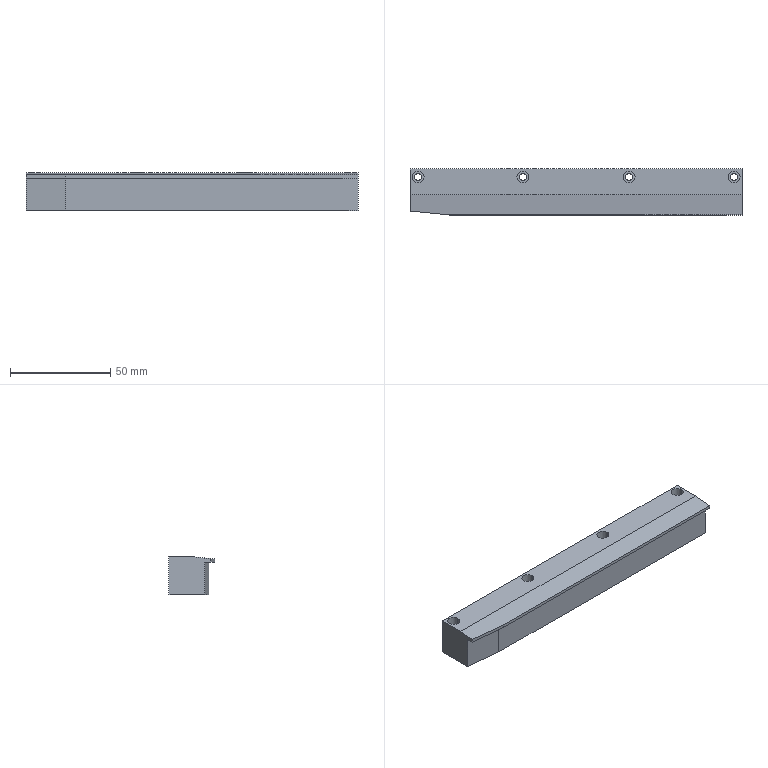Part | SolidWorks | features BaseBody 1 | 1 solid | 31 faces | box 166 x 23 x 19 mm | volume 61656 mm3 | cylinder 16 | plane 15 | commonest cylinder face diameters 3.5 x8 6 x8
STEP:
#1=CARTESIAN_POINT('',(-20.019,-11.953,0.));
#2=VERTEX_POINT('',#1);
#3=CARTESIAN_POINT('',(-23.519,-11.953,0.));
#4=VERTEX_POINT('',#3);
#5=CARTESIAN_POINT('',(-21.769,-11.953,0.));
#6=DIRECTION('',(0.,0.,-1.));
#7=DIRECTION('',(1.,0.,0.));
#8=AXIS2_PLACEMENT_3D('',#5,#6,#7);
#9=CIRCLE('',#8,1.75);
#10=EDGE_CURVE('',#2,#4,#9,.T.);
#11=ORIENTED_EDGE('',*,*,#10,.T.);
#12=CARTESIAN_POINT('',(-23.519,-11.953,9.));
#13=VERTEX_POINT('',#12);
#14=CARTESIAN_POINT('',(-23.519,-11.953,-149.799));
#15=DIRECTION('',(0.,0.,1.));
#16=VECTOR('',#15,1000.);
#17=LINE('',#14,#16);
#18=EDGE_CURVE('',#4,#13,#17,.T.);
#19=ORIENTED_EDGE('',*,*,#18,.T.);
#20=CARTESIAN_POINT('',(-20.019,-11.953,9.));
#21=VERTEX_POINT('',#20);
#22=CARTESIAN_POINT('',(-21.769,-11.953,9.));
#23=DIRECTION('',(0.,0.,-1.));
#24=DIRECTION('',(1.,0.,0.));
#25=AXIS2_PLACEMENT_3D('',#22,#23,#24);
#26=CIRCLE('',#25,1.75);
#27=EDGE_CURVE('',#21,#13,#26,.T.);
#28=ORIENTED_EDGE('',*,*,#27,.F.);
#29=CARTESIAN_POINT('',(-20.019,-11.953,-149.799));
#30=DIRECTION('',(0.,0.,1.));
#31=VECTOR('',#30,1000.);
#32=LINE('',#29,#31);
#33=EDGE_CURVE('',#2,#21,#32,.T.);
#34=ORIENTED_EDGE('',*,*,#33,.F.);
#35=EDGE_LOOP('',(#11,#19,#28,#34));
#36=FACE_OUTER_BOUND('',#35,.T.);
#37=CARTESIAN_POINT('',(-21.769,-11.953,-149.799));
#38=DIRECTION('',(0.,0.,1.));
#39=DIRECTION('',(1.,0.,0.));
#40=AXIS2_PLACEMENT_3D('',#37,#38,#39);
#41=CYLINDRICAL_SURFACE('',#40,1.75);
#42=ADVANCED_FACE('',(#36),#41,.F.);
#43=CARTESIAN_POINT('',(32.481,-11.953,0.));
#44=VERTEX_POINT('',#43);
#45=CARTESIAN_POINT('',(28.981,-11.953,0.));
#46=VERTEX_POINT('',#45);
#47=CARTESIAN_POINT('',(30.731,-11.953,0.));
#48=DIRECTION('',(0.,0.,-1.));
#49=DIRECTION('',(1.,0.,0.));
#50=AXIS2_PLACEMENT_3D('',#47,#48,#49);
#51=CIRCLE('',#50,1.75);
#52=EDGE_CURVE('',#44,#46,#51,.T.);
#53=ORIENTED_EDGE('',*,*,#52,.T.);
#54=CARTESIAN_POINT('',(28.981,-11.953,9.));
#55=VERTEX_POINT('',#54);
#56=CARTESIAN_POINT('',(28.981,-11.953,-149.799));
#57=DIRECTION('',(0.,0.,1.));
#58=VECTOR('',#57,1000.);
#59=LINE('',#56,#58);
#60=EDGE_CURVE('',#46,#55,#59,.T.);
#61=ORIENTED_EDGE('',*,*,#60,.T.);
#62=CARTESIAN_POINT('',(32.481,-11.953,9.));
#63=VERTEX_POINT('',#62);
#64=CARTESIAN_POINT('',(30.731,-11.953,9.));
#65=DIRECTION('',(0.,0.,-1.));
#66=DIRECTION('',(1.,0.,0.));
#67=AXIS2_PLACEMENT_3D('',#64,#65,#66);
#68=CIRCLE('',#67,1.75);
#69=EDGE_CURVE('',#63,#55,#68,.T.);
#70=ORIENTED_EDGE('',*,*,#69,.F.);
#71=CARTESIAN_POINT('',(32.481,-11.953,-149.799));
#72=DIRECTION('',(0.,0.,1.));
#73=VECTOR('',#72,1000.);
#74=LINE('',#71,#73);
#75=EDGE_CURVE('',#44,#63,#74,.T.);
#76=ORIENTED_EDGE('',*,*,#75,.F.);
#77=EDGE_LOOP('',(#53,#61,#70,#76));
#78=FACE_OUTER_BOUND('',#77,.T.);
#79=CARTESIAN_POINT('',(30.731,-11.953,-149.799));
#80=DIRECTION('',(0.,0.,1.));
#81=DIRECTION('',(1.,0.,0.));
#82=AXIS2_PLACEMENT_3D('',#79,#80,#81);
#83=CYLINDRICAL_SURFACE('',#82,1.75);
#84=ADVANCED_FACE('',(#78),#83,.F.);
#85=CARTESIAN_POINT('',(85.481,-11.953,0.));
#86=VERTEX_POINT('',#85);
#87=CARTESIAN_POINT('',(81.981,-11.953,0.));
#88=VERTEX_POINT('',#87);
#89=CARTESIAN_POINT('',(83.731,-11.953,0.));
#90=DIRECTION('',(0.,0.,-1.));
#91=DIRECTION('',(1.,0.,0.));
#92=AXIS2_PLACEMENT_3D('',#89,#90,#91);
#93=CIRCLE('',#92,1.75);
#94=EDGE_CURVE('',#86,#88,#93,.T.);
#95=ORIENTED_EDGE('',*,*,#94,.T.);
#96=CARTESIAN_POINT('',(81.981,-11.953,9.));
#97=VERTEX_POINT('',#96);
#98=CARTESIAN_POINT('',(81.981,-11.953,-149.799));
#99=DIRECTION('',(0.,0.,1.));
#100=VECTOR('',#99,1000.);
#101=LINE('',#98,#100);
#102=EDGE_CURVE('',#88,#97,#101,.T.);
#103=ORIENTED_EDGE('',*,*,#102,.T.);
#104=CARTESIAN_POINT('',(85.481,-11.953,9.));
#105=VERTEX_POINT('',#104);
#106=CARTESIAN_POINT('',(83.731,-11.953,9.));
#107=DIRECTION('',(0.,0.,-1.));
#108=DIRECTION('',(1.,0.,0.));
#109=AXIS2_PLACEMENT_3D('',#106,#107,#108);
#110=CIRCLE('',#109,1.75);
#111=EDGE_CURVE('',#105,#97,#110,.T.);
#112=ORIENTED_EDGE('',*,*,#111,.F.);
#113=CARTESIAN_POINT('',(85.481,-11.953,-149.799));
#114=DIRECTION('',(0.,0.,1.));
#115=VECTOR('',#114,1000.);
#116=LINE('',#113,#115);
#117=EDGE_CURVE('',#86,#105,#116,.T.);
#118=ORIENTED_EDGE('',*,*,#117,.F.);
#119=EDGE_LOOP('',(#95,#103,#112,#118));
#120=FACE_OUTER_BOUND('',#119,.T.);
#121=CARTESIAN_POINT('',(83.731,-11.953,-149.799));
#122=DIRECTION('',(0.,0.,1.));
#123=DIRECTION('',(1.,0.,0.));
#124=AXIS2_PLACEMENT_3D('',#121,#122,#123);
#125=CYLINDRICAL_SURFACE('',#124,1.75);
#126=ADVANCED_FACE('',(#120),#125,.F.);
#127=CARTESIAN_POINT('',(137.981,-11.953,0.));
#128=VERTEX_POINT('',#127);
#129=CARTESIAN_POINT('',(134.481,-11.953,0.));
#130=VERTEX_POINT('',#129);
#131=CARTESIAN_POINT('',(136.231,-11.953,0.));
#132=DIRECTION('',(0.,0.,-1.));
#133=DIRECTION('',(1.,0.,0.));
#134=AXIS2_PLACEMENT_3D('',#131,#132,#133);
#135=CIRCLE('',#134,1.75);
#136=EDGE_CURVE('',#128,#130,#135,.T.);
#137=ORIENTED_EDGE('',*,*,#136,.T.);
#138=CARTESIAN_POINT('',(134.481,-11.953,9.));
#139=VERTEX_POINT('',#138);
#140=CARTESIAN_POINT('',(134.481,-11.953,-149.799));
#141=DIRECTION('',(0.,0.,1.));
#142=VECTOR('',#141,1000.);
#143=LINE('',#140,#142);
#144=EDGE_CURVE('',#130,#139,#143,.T.);
#145=ORIENTED_EDGE('',*,*,#144,.T.);
#146=CARTESIAN_POINT('',(137.981,-11.953,9.));
#147=VERTEX_POINT('',#146);
#148=CARTESIAN_POINT('',(136.231,-11.953,9.));
#149=DIRECTION('',(0.,0.,-1.));
#150=DIRECTION('',(1.,0.,0.));
#151=AXIS2_PLACEMENT_3D('',#148,#149,#150);
#152=CIRCLE('',#151,1.75);
#153=EDGE_CURVE('',#147,#139,#152,.T.);
#154=ORIENTED_EDGE('',*,*,#153,.F.);
#155=CARTESIAN_POINT('',(137.981,-11.953,-149.799));
#156=DIRECTION('',(0.,0.,1.));
#157=VECTOR('',#156,1000.);
#158=LINE('',#155,#157);
#159=EDGE_CURVE('',#128,#147,#158,.T.);
#160=ORIENTED_EDGE('',*,*,#159,.F.);
#161=EDGE_LOOP('',(#137,#145,#154,#160));
#162=FACE_OUTER_BOUND('',#161,.T.);
#163=CARTESIAN_POINT('',(136.231,-11.953,-149.799));
#164=DIRECTION('',(0.,0.,1.));
#165=DIRECTION('',(1.,0.,0.));
#166=AXIS2_PLACEMENT_3D('',#163,#164,#165);
#167=CYLINDRICAL_SURFACE('',#166,1.75);
#168=ADVANCED_FACE('',(#162),#167,.F.);
#169=CARTESIAN_POINT('',(-24.769,-11.953,9.));
#170=VERTEX_POINT('',#169);
#171=CARTESIAN_POINT('',(-18.769,-11.953,9.));
#172=VERTEX_POINT('',#171);
#173=CARTESIAN_POINT('',(-21.769,-11.953,9.));
#174=DIRECTION('',(0.,0.,1.));
#175=DIRECTION('',(1.,0.,0.));
#176=AXIS2_PLACEMENT_3D('',#173,#174,#175);
#177=CIRCLE('',#176,3.);
#178=EDGE_CURVE('',#170,#172,#177,.T.);
#179=ORIENTED_EDGE('',*,*,#178,.F.);
#180=CARTESIAN_POINT('',(-24.769,-11.953,19.));
#181=VERTEX_POINT('',#180);
#182=CARTESIAN_POINT('',(-24.769,-11.953,14.));
#183=DIRECTION('',(0.,0.,1.));
#184=VECTOR('',#183,1000.);
#185=LINE('',#182,#184);
#186=EDGE_CURVE('',#170,#181,#185,.T.);
#187=ORIENTED_EDGE('',*,*,#186,.T.);
#188=CARTESIAN_POINT('',(-18.769,-11.953,19.));
#189=VERTEX_POINT('',#188);
#190=CARTESIAN_POINT('',(-21.769,-11.953,19.));
#191=DIRECTION('',(0.,0.,-1.));
#192=DIRECTION('',(1.,0.,0.));
#193=AXIS2_PLACEMENT_3D('',#190,#191,#192);
#194=CIRCLE('',#193,3.);
#195=EDGE_CURVE('',#189,#181,#194,.T.);
#196=ORIENTED_EDGE('',*,*,#195,.F.);
#197=CARTESIAN_POINT('',(-18.769,-11.953,14.));
#198=DIRECTION('',(0.,0.,1.));
#199=VECTOR('',#198,1000.);
#200=LINE('',#197,#199);
#201=EDGE_CURVE('',#172,#189,#200,.T.);
#202=ORIENTED_EDGE('',*,*,#201,.F.);
#203=EDGE_LOOP('',(#179,#187,#196,#202));
#204=FACE_OUTER_BOUND('',#203,.T.);
#205=CARTESIAN_POINT('',(-21.769,-11.953,14.));
#206=DIRECTION('',(0.,0.,1.));
#207=DIRECTION('',(1.,0.,0.));
#208=AXIS2_PLACEMENT_3D('',#205,#206,#207);
#209=CYLINDRICAL_SURFACE('',#208,3.);
#210=ADVANCED_FACE('',(#204),#209,.F.);
#211=CARTESIAN_POINT('',(27.731,-11.953,9.));
#212=VERTEX_POINT('',#211);
#213=CARTESIAN_POINT('',(33.731,-11.953,9.));
#214=VERTEX_POINT('',#213);
#215=CARTESIAN_POINT('',(30.731,-11.953,9.));
#216=DIRECTION('',(0.,0.,1.));
#217=DIRECTION('',(1.,0.,0.));
#218=AXIS2_PLACEMENT_3D('',#215,#216,#217);
#219=CIRCLE('',#218,3.);
#220=EDGE_CURVE('',#212,#214,#219,.T.);
#221=ORIENTED_EDGE('',*,*,#220,.F.);
#222=CARTESIAN_POINT('',(27.731,-11.953,19.));
#223=VERTEX_POINT('',#222);
#224=CARTESIAN_POINT('',(27.731,-11.953,14.));
#225=DIRECTION('',(0.,0.,1.));
#226=VECTOR('',#225,1000.);
#227=LINE('',#224,#226);
#228=EDGE_CURVE('',#212,#223,#227,.T.);
#229=ORIENTED_EDGE('',*,*,#228,.T.);
#230=CARTESIAN_POINT('',(33.731,-11.953,19.));
#231=VERTEX_POINT('',#230);
#232=CARTESIAN_POINT('',(30.731,-11.953,19.));
#233=DIRECTION('',(0.,0.,-1.));
#234=DIRECTION('',(1.,0.,0.));
#235=AXIS2_PLACEMENT_3D('',#232,#233,#234);
#236=CIRCLE('',#235,3.);
#237=EDGE_CURVE('',#231,#223,#236,.T.);
#238=ORIENTED_EDGE('',*,*,#237,.F.);
#239=CARTESIAN_POINT('',(33.731,-11.953,14.));
#240=DIRECTION('',(0.,0.,1.));
#241=VECTOR('',#240,1000.);
#242=LINE('',#239,#241);
#243=EDGE_CURVE('',#214,#231,#242,.T.);
#244=ORIENTED_EDGE('',*,*,#243,.F.);
#245=EDGE_LOOP('',(#221,#229,#238,#244));
#246=FACE_OUTER_BOUND('',#245,.T.);
#247=CARTESIAN_POINT('',(30.731,-11.953,14.));
#248=DIRECTION('',(0.,0.,1.));
#249=DIRECTION('',(1.,0.,0.));
#250=AXIS2_PLACEMENT_3D('',#247,#248,#249);
#251=CYLINDRICAL_SURFACE('',#250,3.);
#252=ADVANCED_FACE('',(#246),#251,.F.);
#253=CARTESIAN_POINT('',(80.731,-11.953,9.));
#254=VERTEX_POINT('',#253);
#255=CARTESIAN_POINT('',(86.731,-11.953,9.));
#256=VERTEX_POINT('',#255);
#257=CARTESIAN_POINT('',(83.731,-11.953,9.));
#258=DIRECTION('',(0.,0.,1.));
#259=DIRECTION('',(1.,0.,0.));
#260=AXIS2_PLACEMENT_3D('',#257,#258,#259);
#261=CIRCLE('',#260,3.);
#262=EDGE_CURVE('',#254,#256,#261,.T.);
#263=ORIENTED_EDGE('',*,*,#262,.F.);
#264=CARTESIAN_POINT('',(80.731,-11.953,19.));
#265=VERTEX_POINT('',#264);
#266=CARTESIAN_POINT('',(80.731,-11.953,14.));
#267=DIRECTION('',(0.,0.,1.));
#268=VECTOR('',#267,1000.);
#269=LINE('',#266,#268);
#270=EDGE_CURVE('',#254,#265,#269,.T.);
#271=ORIENTED_EDGE('',*,*,#270,.T.);
#272=CARTESIAN_POINT('',(86.731,-11.953,19.));
#273=VERTEX_POINT('',#272);
#274=CARTESIAN_POINT('',(83.731,-11.953,19.));
#275=DIRECTION('',(0.,0.,-1.));
#276=DIRECTION('',(1.,0.,0.));
#277=AXIS2_PLACEMENT_3D('',#274,#275,#276);
#278=CIRCLE('',#277,3.);
#279=EDGE_CURVE('',#273,#265,#278,.T.);
#280=ORIENTED_EDGE('',*,*,#279,.F.);
#281=CARTESIAN_POINT('',(86.731,-11.953,14.));
#282=DIRECTION('',(0.,0.,1.));
#283=VECTOR('',#282,1000.);
#284=LINE('',#281,#283);
#285=EDGE_CURVE('',#256,#273,#284,.T.);
#286=ORIENTED_EDGE('',*,*,#285,.F.);
#287=EDGE_LOOP('',(#263,#271,#280,#286));
#288=FACE_OUTER_BOUND('',#287,.T.);
#289=CARTESIAN_POINT('',(83.731,-11.953,14.));
#290=DIRECTION('',(0.,0.,1.));
#291=DIRECTION('',(1.,0.,0.));
#292=AXIS2_PLACEMENT_3D('',#289,#290,#291);
#293=CYLINDRICAL_SURFACE('',#292,3.);
#294=ADVANCED_FACE('',(#288),#293,.F.);
#295=CARTESIAN_POINT('',(133.231,-11.953,9.));
#296=VERTEX_POINT('',#295);
#297=CARTESIAN_POINT('',(139.231,-11.953,9.));
#298=VERTEX_POINT('',#297);
#299=CARTESIAN_POINT('',(136.231,-11.953,9.));
#300=DIRECTION('',(0.,0.,1.));
#301=DIRECTION('',(1.,0.,0.));
#302=AXIS2_PLACEMENT_3D('',#299,#300,#301);
#303=CIRCLE('',#302,3.);
#304=EDGE_CURVE('',#296,#298,#303,.T.);
#305=ORIENTED_EDGE('',*,*,#304,.F.);
#306=CARTESIAN_POINT('',(133.231,-11.953,19.));
#307=VERTEX_POINT('',#306);
#308=CARTESIAN_POINT('',(133.231,-11.953,14.));
#309=DIRECTION('',(0.,0.,1.));
#310=VECTOR('',#309,1000.);
#311=LINE('',#308,#310);
#312=EDGE_CURVE('',#296,#307,#311,.T.);
#313=ORIENTED_EDGE('',*,*,#312,.T.);
#314=CARTESIAN_POINT('',(139.231,-11.953,19.));
#315=VERTEX_POINT('',#314);
#316=CARTESIAN_POINT('',(136.231,-11.953,19.));
#317=DIRECTION('',(0.,0.,-1.));
#318=DIRECTION('',(1.,0.,0.));
#319=AXIS2_PLACEMENT_3D('',#316,#317,#318);
#320=CIRCLE('',#319,3.);
#321=EDGE_CURVE('',#315,#307,#320,.T.);
#322=ORIENTED_EDGE('',*,*,#321,.F.);
#323=CARTESIAN_POINT('',(139.231,-11.953,14.));
#324=DIRECTION('',(0.,0.,1.));
#325=VECTOR('',#324,1000.);
#326=LINE('',#323,#325);
#327=EDGE_CURVE('',#298,#315,#326,.T.);
#328=ORIENTED_EDGE('',*,*,#327,.F.);
#329=EDGE_LOOP('',(#305,#313,#322,#328));
#330=FACE_OUTER_BOUND('',#329,.T.);
#331=CARTESIAN_POINT('',(136.231,-11.953,14.));
#332=DIRECTION('',(0.,0.,1.));
#333=DIRECTION('',(1.,0.,0.));
#334=AXIS2_PLACEMENT_3D('',#331,#332,#333);
#335=CYLINDRICAL_SURFACE('',#334,3.);
#336=ADVANCED_FACE('',(#330),#335,.F.);
#337=ORIENTED_EDGE('',*,*,#10,.F.);
#338=CARTESIAN_POINT('',(-21.769,-11.953,0.));
#339=DIRECTION('',(0.,0.,-1.));
#340=DIRECTION('',(1.,0.,0.));
#341=AXIS2_PLACEMENT_3D('',#338,#339,#340);
#342=CIRCLE('',#341,1.75);
#343=EDGE_CURVE('',#4,#2,#342,.T.);
#344=ORIENTED_EDGE('',*,*,#343,.F.);
#345=EDGE_LOOP('',(#337,#344));
#346=FACE_BOUND('',#345,.T.);
#347=ORIENTED_EDGE('',*,*,#52,.F.);
#348=CARTESIAN_POINT('',(30.731,-11.953,0.));
#349=DIRECTION('',(0.,0.,-1.));
#350=DIRECTION('',(1.,0.,0.));
#351=AXIS2_PLACEMENT_3D('',#348,#349,#350);
#352=CIRCLE('',#351,1.75);
#353=EDGE_CURVE('',#46,#44,#352,.T.);
#354=ORIENTED_EDGE('',*,*,#353,.F.);
#355=EDGE_LOOP('',(#347,#354));
#356=FACE_BOUND('',#355,.T.);
#357=ORIENTED_EDGE('',*,*,#94,.F.);
#358=CARTESIAN_POINT('',(83.731,-11.953,0.));
#359=DIRECTION('',(0.,0.,-1.));
#360=DIRECTION('',(1.,0.,0.));
#361=AXIS2_PLACEMENT_3D('',#358,#359,#360);
#362=CIRCLE('',#361,1.75);
#363=EDGE_CURVE('',#88,#86,#362,.T.);
#364=ORIENTED_EDGE('',*,*,#363,.F.);
#365=EDGE_LOOP('',(#357,#364));
#366=FACE_BOUND('',#365,.T.);
#367=ORIENTED_EDGE('',*,*,#136,.F.);
#368=CARTESIAN_POINT('',(136.231,-11.953,0.));
#369=DIRECTION('',(0.,0.,-1.));
#370=DIRECTION('',(1.,0.,0.));
#371=AXIS2_PLACEMENT_3D('',#368,#369,#370);
#372=CIRCLE('',#371,1.75);
#373=EDGE_CURVE('',#130,#128,#372,.T.);
#374=ORIENTED_EDGE('',*,*,#373,.F.);
#375=EDGE_LOOP('',(#367,#374));
#376=FACE_BOUND('',#375,.T.);
#377=CARTESIAN_POINT('',(-25.769,-7.953,0.));
#378=VERTEX_POINT('',#377);
#379=CARTESIAN_POINT('',(-25.769,-25.953,0.));
#380=VERTEX_POINT('',#379);
#381=CARTESIAN_POINT('',(-25.769,-19.953,0.));
#382=DIRECTION('',(0.,-1.,0.));
#383=VECTOR('',#382,1000.);
#384=LINE('',#381,#383);
#385=EDGE_CURVE('',#378,#380,#384,.T.);
#386=ORIENTED_EDGE('',*,*,#385,.F.);
#387=CARTESIAN_POINT('',(140.231,-7.953,0.));
#388=VERTEX_POINT('',#387);
#389=CARTESIAN_POINT('',(57.231,-7.953,0.));
#390=DIRECTION('',(-1.,0.,0.));
#391=VECTOR('',#390,1000.);
#392=LINE('',#389,#391);
#393=EDGE_CURVE('',#388,#378,#392,.T.);
#394=ORIENTED_EDGE('',*,*,#393,.F.);
#395=CARTESIAN_POINT('',(140.231,-27.953,0.));
#396=VERTEX_POINT('',#395);
#397=CARTESIAN_POINT('',(140.231,-19.953,0.));
#398=DIRECTION('',(0.,1.,0.));
#399=VECTOR('',#398,1000.);
#400=LINE('',#397,#399);
#401=EDGE_CURVE('',#396,#388,#400,.T.);
#402=ORIENTED_EDGE('',*,*,#401,.F.);
#403=CARTESIAN_POINT('',(-5.769,-27.953,0.));
#404=VERTEX_POINT('',#403);
#405=CARTESIAN_POINT('',(57.231,-27.953,0.));
#406=DIRECTION('',(1.,0.,0.));
#407=VECTOR('',#406,1000.);
#408=LINE('',#405,#407);
#409=EDGE_CURVE('',#404,#396,#408,.T.);
#410=ORIENTED_EDGE('',*,*,#409,.F.);
#411=CARTESIAN_POINT('',(-25.769,-25.953,0.));
#412=DIRECTION('',(0.995,-0.0995,0.));
#413=VECTOR('',#412,1000.);
#414=LINE('',#411,#413);
#415=EDGE_CURVE('',#380,#404,#414,.T.);
#416=ORIENTED_EDGE('',*,*,#415,.F.);
#417=EDGE_LOOP('',(#386,#394,#402,#410,#416));
#418=FACE_OUTER_BOUND('',#417,.T.);
#419=CARTESIAN_POINT('',(57.231,-19.953,0.));
#420=DIRECTION('',(0.,0.,1.));
#421=DIRECTION('',(1.,0.,0.));
#422=AXIS2_PLACEMENT_3D('',#419,#420,#421);
#423=PLANE('',#422);
#424=ADVANCED_FACE('',(#346,#356,#366,#376,#418),#423,.F.);
#425=ORIENTED_EDGE('',*,*,#18,.F.);
#426=ORIENTED_EDGE('',*,*,#343,.T.);
#427=ORIENTED_EDGE('',*,*,#33,.T.);
#428=CARTESIAN_POINT('',(-21.769,-11.953,9.));
#429=DIRECTION('',(0.,0.,-1.));
#430=DIRECTION('',(1.,0.,0.));
#431=AXIS2_PLACEMENT_3D('',#428,#429,#430);
#432=CIRCLE('',#431,1.75);
#433=EDGE_CURVE('',#13,#21,#432,.T.);
#434=ORIENTED_EDGE('',*,*,#433,.F.);
#435=EDGE_LOOP('',(#425,#426,#427,#434));
#436=FACE_OUTER_BOUND('',#435,.T.);
#437=CARTESIAN_POINT('',(-21.769,-11.953,-149.799));
#438=DIRECTION('',(0.,0.,1.));
#439=DIRECTION('',(1.,0.,0.));
#440=AXIS2_PLACEMENT_3D('',#437,#438,#439);
#441=CYLINDRICAL_SURFACE('',#440,1.75);
#442=ADVANCED_FACE('',(#436),#441,.F.);
#443=ORIENTED_EDGE('',*,*,#60,.F.);
#444=ORIENTED_EDGE('',*,*,#353,.T.);
#445=ORIENTED_EDGE('',*,*,#75,.T.);
#446=CARTESIAN_POINT('',(30.731,-11.953,9.));
#447=DIRECTION('',(0.,0.,-1.));
#448=DIRECTION('',(1.,0.,0.));
#449=AXIS2_PLACEMENT_3D('',#446,#447,#448);
#450=CIRCLE('',#449,1.75);
#451=EDGE_CURVE('',#55,#63,#450,.T.);
#452=ORIENTED_EDGE('',*,*,#451,.F.);
#453=EDGE_LOOP('',(#443,#444,#445,#452));
#454=FACE_OUTER_BOUND('',#453,.T.);
#455=CARTESIAN_POINT('',(30.731,-11.953,-149.799));
#456=DIRECTION('',(0.,0.,1.));
#457=DIRECTION('',(1.,0.,0.));
#458=AXIS2_PLACEMENT_3D('',#455,#456,#457);
#459=CYLINDRICAL_SURFACE('',#458,1.75);
#460=ADVANCED_FACE('',(#454),#459,.F.);
#461=ORIENTED_EDGE('',*,*,#102,.F.);
#462=ORIENTED_EDGE('',*,*,#363,.T.);
#463=ORIENTED_EDGE('',*,*,#117,.T.);
#464=CARTESIAN_POINT('',(83.731,-11.953,9.));
#465=DIRECTION('',(0.,0.,-1.));
#466=DIRECTION('',(1.,0.,0.));
#467=AXIS2_PLACEMENT_3D('',#464,#465,#466);
#468=CIRCLE('',#467,1.75);
#469=EDGE_CURVE('',#97,#105,#468,.T.);
#470=ORIENTED_EDGE('',*,*,#469,.F.);
#471=EDGE_LOOP('',(#461,#462,#463,#470));
#472=FACE_OUTER_BOUND('',#471,.T.);
#473=CARTESIAN_POINT('',(83.731,-11.953,-149.799));
#474=DIRECTION('',(0.,0.,1.));
#475=DIRECTION('',(1.,0.,0.));
#476=AXIS2_PLACEMENT_3D('',#473,#474,#475);
#477=CYLINDRICAL_SURFACE('',#476,1.75);
#478=ADVANCED_FACE('',(#472),#477,.F.);
#479=ORIENTED_EDGE('',*,*,#144,.F.);
#480=ORIENTED_EDGE('',*,*,#373,.T.);
#481=ORIENTED_EDGE('',*,*,#159,.T.);
#482=CARTESIAN_POINT('',(136.231,-11.953,9.));
#483=DIRECTION('',(0.,0.,-1.));
#484=DIRECTION('',(1.,0.,0.));
#485=AXIS2_PLACEMENT_3D('',#482,#483,#484);
#486=CIRCLE('',#485,1.75);
#487=EDGE_CURVE('',#139,#147,#486,.T.);
#488=ORIENTED_EDGE('',*,*,#487,.F.);
#489=EDGE_LOOP('',(#479,#480,#481,#488));
#490=FACE_OUTER_BOUND('',#489,.T.);
#491=CARTESIAN_POINT('',(136.231,-11.953,-149.799));
#492=DIRECTION('',(0.,0.,1.));
#493=DIRECTION('',(1.,0.,0.));
#494=AXIS2_PLACEMENT_3D('',#491,#492,#493);
#495=CYLINDRICAL_SURFACE('',#494,1.75);
#496=ADVANCED_FACE('',(#490),#495,.F.);
#497=CARTESIAN_POINT('',(-5.769,-27.953,16.5));
#498=VERTEX_POINT('',#497);
#499=CARTESIAN_POINT('',(-25.769,-25.953,16.5));
#500=VERTEX_POINT('',#499);
#501=CARTESIAN_POINT('',(-15.769,-26.953,16.5));
#502=DIRECTION('',(-0.995,0.0995,0.));
#503=VECTOR('',#502,1000.);
#504=LINE('',#501,#503);
#505=EDGE_CURVE('',#498,#500,#504,.T.);
#506=ORIENTED_EDGE('',*,*,#505,.T.);
#507=CARTESIAN_POINT('',(-25.769,-25.953,0.));
#508=DIRECTION('',(0.,0.,-1.));
#509=VECTOR('',#508,1000.);
#510=LINE('',#507,#509);
#511=EDGE_CURVE('',#500,#380,#510,.T.);
#512=ORIENTED_EDGE('',*,*,#511,.T.);
#513=ORIENTED_EDGE('',*,*,#415,.T.);
#514=CARTESIAN_POINT('',(-5.769,-27.953,0.));
#515=DIRECTION('',(0.,0.,1.));
#516=VECTOR('',#515,1000.);
#517=LINE('',#514,#516);
#518=EDGE_CURVE('',#404,#498,#517,.T.);
#519=ORIENTED_EDGE('',*,*,#518,.T.);
#520=EDGE_LOOP('',(#506,#512,#513,#519));
#521=FACE_OUTER_BOUND('',#520,.T.);
#522=CARTESIAN_POINT('',(-15.769,-26.953,0.));
#523=DIRECTION('',(-0.0995,-0.995,0.));
#524=DIRECTION('',(0.995,-0.0995,0.));
#525=AXIS2_PLACEMENT_3D('',#522,#523,#524);
#526=PLANE('',#525);
#527=ADVANCED_FACE('',(#521),#526,.T.);
#528=ORIENTED_EDGE('',*,*,#511,.F.);
#529=CARTESIAN_POINT('',(-25.769,-28.953,16.5));
#530=VERTEX_POINT('',#529);
#531=CARTESIAN_POINT('',(-25.769,-31.953,16.5));
#532=DIRECTION('',(0.,-1.,0.));
#533=VECTOR('',#532,1000.);
#534=LINE('',#531,#533);
#535=EDGE_CURVE('',#500,#530,#534,.T.);
#536=ORIENTED_EDGE('',*,*,#535,.T.);
#537=CARTESIAN_POINT('',(-25.769,-28.953,18.2));
#538=VERTEX_POINT('',#537);
#539=CARTESIAN_POINT('',(-25.769,-28.953,8.875));
#540=DIRECTION('',(0.,0.,-1.));
#541=VECTOR('',#540,1000.);
#542=LINE('',#539,#541);
#543=EDGE_CURVE('',#538,#530,#542,.T.);
#544=ORIENTED_EDGE('',*,*,#543,.F.);
#545=CARTESIAN_POINT('',(-25.769,-20.953,19.));
#546=VERTEX_POINT('',#545);
#547=CARTESIAN_POINT('',(-25.769,-28.953,18.2));
#548=DIRECTION('',(0.,0.995,0.0995));
#549=VECTOR('',#548,1000.);
#550=LINE('',#547,#549);
#551=EDGE_CURVE('',#538,#546,#550,.T.);
#552=ORIENTED_EDGE('',*,*,#551,.T.);
#553=CARTESIAN_POINT('',(-25.769,-7.953,19.));
#554=VERTEX_POINT('',#553);
#555=CARTESIAN_POINT('',(-25.769,-31.953,19.));
#556=DIRECTION('',(0.,1.,0.));
#557=VECTOR('',#556,1000.);
#558=LINE('',#555,#557);
#559=EDGE_CURVE('',#546,#554,#558,.T.);
#560=ORIENTED_EDGE('',*,*,#559,.T.);
#561=CARTESIAN_POINT('',(-25.769,-7.953,0.));
#562=DIRECTION('',(0.,0.,-1.));
#563=VECTOR('',#562,1000.);
#564=LINE('',#561,#563);
#565=EDGE_CURVE('',#554,#378,#564,.T.);
#566=ORIENTED_EDGE('',*,*,#565,.T.);
#567=ORIENTED_EDGE('',*,*,#385,.T.);
#568=EDGE_LOOP('',(#528,#536,#544,#552,#560,#566,#567));
#569=FACE_OUTER_BOUND('',#568,.T.);
#570=CARTESIAN_POINT('',(-25.769,-31.953,0.));
#571=DIRECTION('',(-1.,0.,0.));
#572=DIRECTION('',(0.,0.,1.));
#573=AXIS2_PLACEMENT_3D('',#570,#571,#572);
#574=PLANE('',#573);
#575=ADVANCED_FACE('',(#569),#574,.T.);
#576=ORIENTED_EDGE('',*,*,#393,.T.);
#577=ORIENTED_EDGE('',*,*,#565,.F.);
#578=CARTESIAN_POINT('',(140.231,-7.953,19.));
#579=VERTEX_POINT('',#578);
#580=CARTESIAN_POINT('',(-25.769,-7.953,19.));
#581=DIRECTION('',(1.,0.,0.));
#582=VECTOR('',#581,1000.);
#583=LINE('',#580,#582);
#584=EDGE_CURVE('',#554,#579,#583,.T.);
#585=ORIENTED_EDGE('',*,*,#584,.T.);
#586=CARTESIAN_POINT('',(140.231,-7.953,0.));
#587=DIRECTION('',(0.,0.,-1.));
#588=VECTOR('',#587,1000.);
#589=LINE('',#586,#588);
#590=EDGE_CURVE('',#579,#388,#589,.T.);
#591=ORIENTED_EDGE('',*,*,#590,.T.);
#592=EDGE_LOOP('',(#576,#577,#585,#591));
#593=FACE_OUTER_BOUND('',#592,.T.);
#594=CARTESIAN_POINT('',(-25.769,-7.953,0.));
#595=DIRECTION('',(0.,1.,0.));
#596=DIRECTION('',(0.,0.,1.));
#597=AXIS2_PLACEMENT_3D('',#594,#595,#596);
#598=PLANE('',#597);
#599=ADVANCED_FACE('',(#593),#598,.T.);
#600=ORIENTED_EDGE('',*,*,#590,.F.);
#601=CARTESIAN_POINT('',(140.231,-20.953,19.));
#602=VERTEX_POINT('',#601);
#603=CARTESIAN_POINT('',(140.231,-7.953,19.));
#604=DIRECTION('',(0.,-1.,0.));
#605=VECTOR('',#604,1000.);
#606=LINE('',#603,#605);
#607=EDGE_CURVE('',#579,#602,#606,.T.);
#608=ORIENTED_EDGE('',*,*,#607,.T.);
#609=CARTESIAN_POINT('',(140.231,-30.953,18.));
#610=VERTEX_POINT('',#609);
#611=CARTESIAN_POINT('',(140.231,-20.953,19.));
#612=DIRECTION('',(0.,-0.995,-0.0995));
#613=VECTOR('',#612,1000.);
#614=LINE('',#611,#613);
#615=EDGE_CURVE('',#602,#610,#614,.T.);
#616=ORIENTED_EDGE('',*,*,#615,.T.);
#617=CARTESIAN_POINT('',(140.231,-30.953,16.5));
#618=VERTEX_POINT('',#617);
#619=CARTESIAN_POINT('',(140.231,-30.953,17.75));
#620=DIRECTION('',(0.,0.,-1.));
#621=VECTOR('',#620,1000.);
#622=LINE('',#619,#621);
#623=EDGE_CURVE('',#610,#618,#622,.T.);
#624=ORIENTED_EDGE('',*,*,#623,.T.);
#625=CARTESIAN_POINT('',(140.231,-27.953,16.5));
#626=VERTEX_POINT('',#625);
#627=CARTESIAN_POINT('',(140.231,-7.953,16.5));
#628=DIRECTION('',(0.,1.,0.));
#629=VECTOR('',#628,1000.);
#630=LINE('',#627,#629);
#631=EDGE_CURVE('',#618,#626,#630,.T.);
#632=ORIENTED_EDGE('',*,*,#631,.T.);
#633=CARTESIAN_POINT('',(140.231,-27.953,0.));
#634=DIRECTION('',(0.,0.,-1.));
#635=VECTOR('',#634,1000.);
#636=LINE('',#633,#635);
#637=EDGE_CURVE('',#626,#396,#636,.T.);
#638=ORIENTED_EDGE('',*,*,#637,.T.);
#639=ORIENTED_EDGE('',*,*,#401,.T.);
#640=EDGE_LOOP('',(#600,#608,#616,#624,#632,#638,#639));
#641=FACE_OUTER_BOUND('',#640,.T.);
#642=CARTESIAN_POINT('',(140.231,-7.953,0.));
#643=DIRECTION('',(1.,0.,0.));
#644=DIRECTION('',(0.,0.,-1.));
#645=AXIS2_PLACEMENT_3D('',#642,#643,#644);
#646=PLANE('',#645);
#647=ADVANCED_FACE('',(#641),#646,.T.);
#648=ORIENTED_EDGE('',*,*,#409,.T.);
#649=ORIENTED_EDGE('',*,*,#637,.F.);
#650=CARTESIAN_POINT('',(-25.769,-27.953,16.5));
#651=DIRECTION('',(1.,0.,0.));
#652=VECTOR('',#651,1000.);
#653=LINE('',#650,#652);
#654=EDGE_CURVE('',#498,#626,#653,.T.);
#655=ORIENTED_EDGE('',*,*,#654,.F.);
#656=ORIENTED_EDGE('',*,*,#518,.F.);
#657=EDGE_LOOP('',(#648,#649,#655,#656));
#658=FACE_OUTER_BOUND('',#657,.T.);
#659=CARTESIAN_POINT('',(-25.769,-27.953,0.));
#660=DIRECTION('',(0.,1.,0.));
#661=DIRECTION('',(0.,0.,1.));
#662=AXIS2_PLACEMENT_3D('',#659,#660,#661);
#663=PLANE('',#662);
#664=ADVANCED_FACE('',(#658),#663,.F.);
#665=ORIENTED_EDGE('',*,*,#27,.T.);
#666=ORIENTED_EDGE('',*,*,#433,.T.);
#667=EDGE_LOOP('',(#665,#666));
#668=FACE_BOUND('',#667,.T.);
#669=CARTESIAN_POINT('',(-21.769,-11.953,9.));
#670=DIRECTION('',(0.,0.,1.));
#671=DIRECTION('',(1.,0.,0.));
#672=AXIS2_PLACEMENT_3D('',#669,#670,#671);
#673=CIRCLE('',#672,3.);
#674=EDGE_CURVE('',#172,#170,#673,.T.);
#675=ORIENTED_EDGE('',*,*,#674,.T.);
#676=ORIENTED_EDGE('',*,*,#178,.T.);
#677=EDGE_LOOP('',(#675,#676));
#678=FACE_OUTER_BOUND('',#677,.T.);
#679=CARTESIAN_POINT('',(-21.769,-11.953,9.));
#680=DIRECTION('',(0.,0.,1.));
#681=DIRECTION('',(1.,0.,0.));
#682=AXIS2_PLACEMENT_3D('',#679,#680,#681);
#683=PLANE('',#682);
#684=ADVANCED_FACE('',(#668,#678),#683,.T.);
#685=ORIENTED_EDGE('',*,*,#69,.T.);
#686=ORIENTED_EDGE('',*,*,#451,.T.);
#687=EDGE_LOOP('',(#685,#686));
#688=FACE_BOUND('',#687,.T.);
#689=CARTESIAN_POINT('',(30.731,-11.953,9.));
#690=DIRECTION('',(0.,0.,1.));
#691=DIRECTION('',(1.,0.,0.));
#692=AXIS2_PLACEMENT_3D('',#689,#690,#691);
#693=CIRCLE('',#692,3.);
#694=EDGE_CURVE('',#214,#212,#693,.T.);
#695=ORIENTED_EDGE('',*,*,#694,.T.);
#696=ORIENTED_EDGE('',*,*,#220,.T.);
#697=EDGE_LOOP('',(#695,#696));
#698=FACE_OUTER_BOUND('',#697,.T.);
#699=CARTESIAN_POINT('',(30.731,-11.953,9.));
#700=DIRECTION('',(0.,0.,1.));
#701=DIRECTION('',(1.,0.,0.));
#702=AXIS2_PLACEMENT_3D('',#699,#700,#701);
#703=PLANE('',#702);
#704=ADVANCED_FACE('',(#688,#698),#703,.T.);
#705=ORIENTED_EDGE('',*,*,#111,.T.);
#706=ORIENTED_EDGE('',*,*,#469,.T.);
#707=EDGE_LOOP('',(#705,#706));
#708=FACE_BOUND('',#707,.T.);
#709=CARTESIAN_POINT('',(83.731,-11.953,9.));
#710=DIRECTION('',(0.,0.,1.));
#711=DIRECTION('',(1.,0.,0.));
#712=AXIS2_PLACEMENT_3D('',#709,#710,#711);
#713=CIRCLE('',#712,3.);
#714=EDGE_CURVE('',#256,#254,#713,.T.);
#715=ORIENTED_EDGE('',*,*,#714,.T.);
#716=ORIENTED_EDGE('',*,*,#262,.T.);
#717=EDGE_LOOP('',(#715,#716));
#718=FACE_OUTER_BOUND('',#717,.T.);
#719=CARTESIAN_POINT('',(83.731,-11.953,9.));
#720=DIRECTION('',(0.,0.,1.));
#721=DIRECTION('',(1.,0.,0.));
#722=AXIS2_PLACEMENT_3D('',#719,#720,#721);
#723=PLANE('',#722);
#724=ADVANCED_FACE('',(#708,#718),#723,.T.);
#725=ORIENTED_EDGE('',*,*,#153,.T.);
#726=ORIENTED_EDGE('',*,*,#487,.T.);
#727=EDGE_LOOP('',(#725,#726));
#728=FACE_BOUND('',#727,.T.);
#729=CARTESIAN_POINT('',(136.231,-11.953,9.));
#730=DIRECTION('',(0.,0.,1.));
#731=DIRECTION('',(1.,0.,0.));
#732=AXIS2_PLACEMENT_3D('',#729,#730,#731);
#733=CIRCLE('',#732,3.);
#734=EDGE_CURVE('',#298,#296,#733,.T.);
#735=ORIENTED_EDGE('',*,*,#734,.T.);
#736=ORIENTED_EDGE('',*,*,#304,.T.);
#737=EDGE_LOOP('',(#735,#736));
#738=FACE_OUTER_BOUND('',#737,.T.);
#739=CARTESIAN_POINT('',(136.231,-11.953,9.));
#740=DIRECTION('',(0.,0.,1.));
#741=DIRECTION('',(1.,0.,0.));
#742=AXIS2_PLACEMENT_3D('',#739,#740,#741);
#743=PLANE('',#742);
#744=ADVANCED_FACE('',(#728,#738),#743,.T.);
#745=ORIENTED_EDGE('',*,*,#535,.F.);
#746=ORIENTED_EDGE('',*,*,#505,.F.);
#747=ORIENTED_EDGE('',*,*,#654,.T.);
#748=ORIENTED_EDGE('',*,*,#631,.F.);
#749=CARTESIAN_POINT('',(-5.769,-30.953,16.5));
#750=VERTEX_POINT('',#749);
#751=CARTESIAN_POINT('',(57.231,-30.953,16.5));
#752=DIRECTION('',(1.,0.,0.));
#753=VECTOR('',#752,1000.);
#754=LINE('',#751,#753);
#755=EDGE_CURVE('',#750,#618,#754,.T.);
#756=ORIENTED_EDGE('',*,*,#755,.F.);
#757=CARTESIAN_POINT('',(-25.769,-28.953,16.5));
#758=DIRECTION('',(0.995,-0.0995,0.));
#759=VECTOR('',#758,1000.);
#760=LINE('',#757,#759);
#761=EDGE_CURVE('',#530,#750,#760,.T.);
#762=ORIENTED_EDGE('',*,*,#761,.F.);
#763=EDGE_LOOP('',(#745,#746,#747,#748,#756,#762));
#764=FACE_OUTER_BOUND('',#763,.T.);
#765=CARTESIAN_POINT('',(57.231,-29.953,16.5));
#766=DIRECTION('',(0.,0.,1.));
#767=DIRECTION('',(1.,0.,0.));
#768=AXIS2_PLACEMENT_3D('',#765,#766,#767);
#769=PLANE('',#768);
#770=ADVANCED_FACE('',(#764),#769,.F.);
#771=ORIENTED_EDGE('',*,*,#195,.T.);
#772=CARTESIAN_POINT('',(-21.769,-11.953,19.));
#773=DIRECTION('',(0.,0.,-1.));
#774=DIRECTION('',(1.,0.,0.));
#775=AXIS2_PLACEMENT_3D('',#772,#773,#774);
#776=CIRCLE('',#775,3.);
#777=EDGE_CURVE('',#181,#189,#776,.T.);
#778=ORIENTED_EDGE('',*,*,#777,.T.);
#779=EDGE_LOOP('',(#771,#778));
#780=FACE_BOUND('',#779,.T.);
#781=ORIENTED_EDGE('',*,*,#237,.T.);
#782=CARTESIAN_POINT('',(30.731,-11.953,19.));
#783=DIRECTION('',(0.,0.,-1.));
#784=DIRECTION('',(1.,0.,0.));
#785=AXIS2_PLACEMENT_3D('',#782,#783,#784);
#786=CIRCLE('',#785,3.);
#787=EDGE_CURVE('',#223,#231,#786,.T.);
#788=ORIENTED_EDGE('',*,*,#787,.T.);
#789=EDGE_LOOP('',(#781,#788));
#790=FACE_BOUND('',#789,.T.);
#791=ORIENTED_EDGE('',*,*,#279,.T.);
#792=CARTESIAN_POINT('',(83.731,-11.953,19.));
#793=DIRECTION('',(0.,0.,-1.));
#794=DIRECTION('',(1.,0.,0.));
#795=AXIS2_PLACEMENT_3D('',#792,#793,#794);
#796=CIRCLE('',#795,3.);
#797=EDGE_CURVE('',#265,#273,#796,.T.);
#798=ORIENTED_EDGE('',*,*,#797,.T.);
#799=EDGE_LOOP('',(#791,#798));
#800=FACE_BOUND('',#799,.T.);
#801=ORIENTED_EDGE('',*,*,#321,.T.);
#802=CARTESIAN_POINT('',(136.231,-11.953,19.));
#803=DIRECTION('',(0.,0.,-1.));
#804=DIRECTION('',(1.,0.,0.));
#805=AXIS2_PLACEMENT_3D('',#802,#803,#804);
#806=CIRCLE('',#805,3.);
#807=EDGE_CURVE('',#307,#315,#806,.T.);
#808=ORIENTED_EDGE('',*,*,#807,.T.);
#809=EDGE_LOOP('',(#801,#808));
#810=FACE_BOUND('',#809,.T.);
#811=ORIENTED_EDGE('',*,*,#584,.F.);
#812=ORIENTED_EDGE('',*,*,#559,.F.);
#813=CARTESIAN_POINT('',(57.231,-20.953,19.));
#814=DIRECTION('',(1.,0.,0.));
#815=VECTOR('',#814,1000.);
#816=LINE('',#813,#815);
#817=EDGE_CURVE('',#546,#602,#816,.T.);
#818=ORIENTED_EDGE('',*,*,#817,.T.);
#819=ORIENTED_EDGE('',*,*,#607,.F.);
#820=EDGE_LOOP('',(#811,#812,#818,#819));
#821=FACE_OUTER_BOUND('',#820,.T.);
#822=CARTESIAN_POINT('',(57.231,-19.953,19.));
#823=DIRECTION('',(0.,0.,1.));
#824=DIRECTION('',(1.,0.,0.));
#825=AXIS2_PLACEMENT_3D('',#822,#823,#824);
#826=PLANE('',#825);
#827=ADVANCED_FACE('',(#780,#790,#800,#810,#821),#826,.T.);
#828=ORIENTED_EDGE('',*,*,#817,.F.);
#829=ORIENTED_EDGE('',*,*,#551,.F.);
#830=CARTESIAN_POINT('',(-5.769,-30.953,18.));
#831=VERTEX_POINT('',#830);
#832=CARTESIAN_POINT('',(-25.769,-28.953,18.2));
#833=DIRECTION('',(0.995,-0.0995,-0.00995));
#834=VECTOR('',#833,1000.);
#835=LINE('',#832,#834);
#836=EDGE_CURVE('',#538,#831,#835,.T.);
#837=ORIENTED_EDGE('',*,*,#836,.T.);
#838=CARTESIAN_POINT('',(57.231,-30.953,18.));
#839=DIRECTION('',(1.,0.,0.));
#840=VECTOR('',#839,1000.);
#841=LINE('',#838,#840);
#842=EDGE_CURVE('',#831,#610,#841,.T.);
#843=ORIENTED_EDGE('',*,*,#842,.T.);
#844=ORIENTED_EDGE('',*,*,#615,.F.);
#845=EDGE_LOOP('',(#828,#829,#837,#843,#844));
#846=FACE_OUTER_BOUND('',#845,.T.);
#847=CARTESIAN_POINT('',(57.231,-25.953,18.5));
#848=DIRECTION('',(0.,-0.0995,0.995));
#849=DIRECTION('',(0.,-0.995,-0.0995));
#850=AXIS2_PLACEMENT_3D('',#847,#848,#849);
#851=PLANE('',#850);
#852=ADVANCED_FACE('',(#846),#851,.T.);
#853=ORIENTED_EDGE('',*,*,#186,.F.);
#854=ORIENTED_EDGE('',*,*,#674,.F.);
#855=ORIENTED_EDGE('',*,*,#201,.T.);
#856=ORIENTED_EDGE('',*,*,#777,.F.);
#857=EDGE_LOOP('',(#853,#854,#855,#856));
#858=FACE_OUTER_BOUND('',#857,.T.);
#859=CARTESIAN_POINT('',(-21.769,-11.953,14.));
#860=DIRECTION('',(0.,0.,1.));
#861=DIRECTION('',(1.,0.,0.));
#862=AXIS2_PLACEMENT_3D('',#859,#860,#861);
#863=CYLINDRICAL_SURFACE('',#862,3.);
#864=ADVANCED_FACE('',(#858),#863,.F.);
#865=ORIENTED_EDGE('',*,*,#228,.F.);
#866=ORIENTED_EDGE('',*,*,#694,.F.);
#867=ORIENTED_EDGE('',*,*,#243,.T.);
#868=ORIENTED_EDGE('',*,*,#787,.F.);
#869=EDGE_LOOP('',(#865,#866,#867,#868));
#870=FACE_OUTER_BOUND('',#869,.T.);
#871=CARTESIAN_POINT('',(30.731,-11.953,14.));
#872=DIRECTION('',(0.,0.,1.));
#873=DIRECTION('',(1.,0.,0.));
#874=AXIS2_PLACEMENT_3D('',#871,#872,#873);
#875=CYLINDRICAL_SURFACE('',#874,3.);
#876=ADVANCED_FACE('',(#870),#875,.F.);
#877=ORIENTED_EDGE('',*,*,#270,.F.);
#878=ORIENTED_EDGE('',*,*,#714,.F.);
#879=ORIENTED_EDGE('',*,*,#285,.T.);
#880=ORIENTED_EDGE('',*,*,#797,.F.);
#881=EDGE_LOOP('',(#877,#878,#879,#880));
#882=FACE_OUTER_BOUND('',#881,.T.);
#883=CARTESIAN_POINT('',(83.731,-11.953,14.));
#884=DIRECTION('',(0.,0.,1.));
#885=DIRECTION('',(1.,0.,0.));
#886=AXIS2_PLACEMENT_3D('',#883,#884,#885);
#887=CYLINDRICAL_SURFACE('',#886,3.);
#888=ADVANCED_FACE('',(#882),#887,.F.);
#889=ORIENTED_EDGE('',*,*,#312,.F.);
#890=ORIENTED_EDGE('',*,*,#734,.F.);
#891=ORIENTED_EDGE('',*,*,#327,.T.);
#892=ORIENTED_EDGE('',*,*,#807,.F.);
#893=EDGE_LOOP('',(#889,#890,#891,#892));
#894=FACE_OUTER_BOUND('',#893,.T.);
#895=CARTESIAN_POINT('',(136.231,-11.953,14.));
#896=DIRECTION('',(0.,0.,1.));
#897=DIRECTION('',(1.,0.,0.));
#898=AXIS2_PLACEMENT_3D('',#895,#896,#897);
#899=CYLINDRICAL_SURFACE('',#898,3.);
#900=ADVANCED_FACE('',(#894),#899,.F.);
#901=ORIENTED_EDGE('',*,*,#761,.T.);
#902=CARTESIAN_POINT('',(-5.769,-30.953,8.875));
#903=DIRECTION('',(0.,0.,1.));
#904=VECTOR('',#903,1000.);
#905=LINE('',#902,#904);
#906=EDGE_CURVE('',#750,#831,#905,.T.);
#907=ORIENTED_EDGE('',*,*,#906,.T.);
#908=ORIENTED_EDGE('',*,*,#836,.F.);
#909=ORIENTED_EDGE('',*,*,#543,.T.);
#910=EDGE_LOOP('',(#901,#907,#908,#909));
#911=FACE_OUTER_BOUND('',#910,.T.);
#912=CARTESIAN_POINT('',(-15.769,-29.953,8.875));
#913=DIRECTION('',(-0.0995,-0.995,0.));
#914=DIRECTION('',(0.995,-0.0995,0.));
#915=AXIS2_PLACEMENT_3D('',#912,#913,#914);
#916=PLANE('',#915);
#917=ADVANCED_FACE('',(#911),#916,.T.);
#918=ORIENTED_EDGE('',*,*,#755,.T.);
#919=ORIENTED_EDGE('',*,*,#623,.F.);
#920=ORIENTED_EDGE('',*,*,#842,.F.);
#921=ORIENTED_EDGE('',*,*,#906,.F.);
#922=EDGE_LOOP('',(#918,#919,#920,#921));
#923=FACE_OUTER_BOUND('',#922,.T.);
#924=CARTESIAN_POINT('',(57.231,-30.953,17.75));
#925=DIRECTION('',(0.,1.,0.));
#926=DIRECTION('',(0.,0.,1.));
#927=AXIS2_PLACEMENT_3D('',#924,#925,#926);
#928=PLANE('',#927);
#929=ADVANCED_FACE('',(#923),#928,.F.);
#930=CLOSED_SHELL('',(#42,#84,#126,#168,#210,#252,#294,#336,#424,#442,#460,#478,#496,#527,#575,#599,#647,#664,#684,#704,#724,#744,#770,#827,#852,#864,#876,#888,#900,#917,#929));
#931=MANIFOLD_SOLID_BREP('',#930);
#932=CARTESIAN_POINT('',(0.,0.,0.));
#933=DIRECTION('',(0.,0.,1.));
#934=DIRECTION('',(1.,0.,0.));
#935=AXIS2_PLACEMENT_3D('',#932,#933,#934);
#936=(LENGTH_UNIT()NAMED_UNIT(*)SI_UNIT(.MILLI.,.METRE.));
#937=UNCERTAINTY_MEASURE_WITH_UNIT(LENGTH_MEASURE(0.00001),#936,'','');
#938=(NAMED_UNIT(*)PLANE_ANGLE_UNIT()SI_UNIT($,.RADIAN.));
#939=(NAMED_UNIT(*)SI_UNIT($,.STERADIAN.)SOLID_ANGLE_UNIT());
#940=(GEOMETRIC_REPRESENTATION_CONTEXT(3)GLOBAL_UNCERTAINTY_ASSIGNED_CONTEXT((#937))GLOBAL_UNIT_ASSIGNED_CONTEXT((#936,#938,#939))REPRESENTATION_CONTEXT('',''));
#941=ADVANCED_BREP_SHAPE_REPRESENTATION('',(#931,#935),#940);